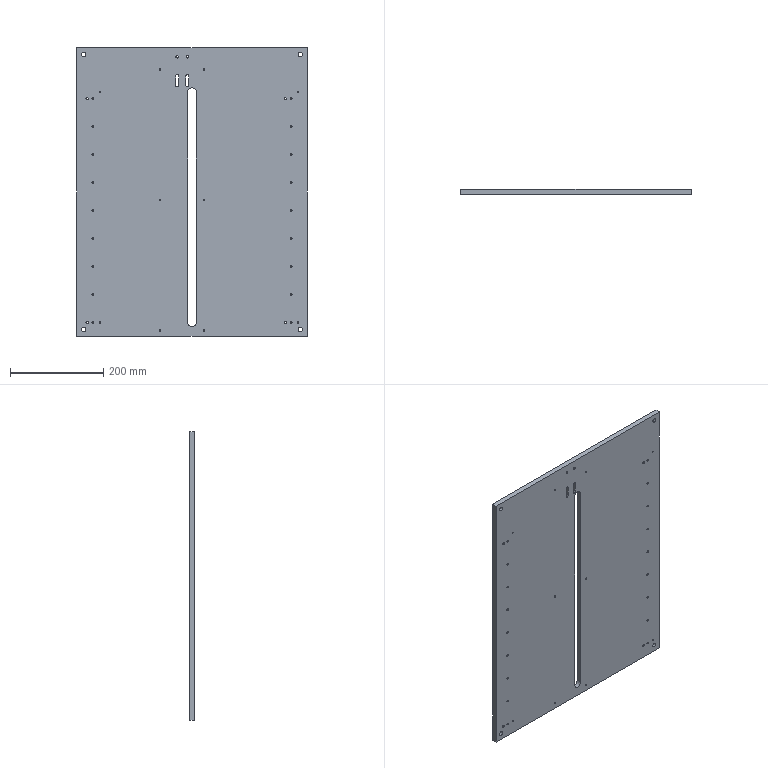Part | STEP file | 0243_210_Plate | 1 solid | 97 faces | box 495 x 10 x 620 mm | volume 2967020 mm3 | cylinder 85 | plane 12 | commonest cylinder face diameters 4.2 x36 3.3 x20 5 x12 9 x8 6.5 x6 18 x3